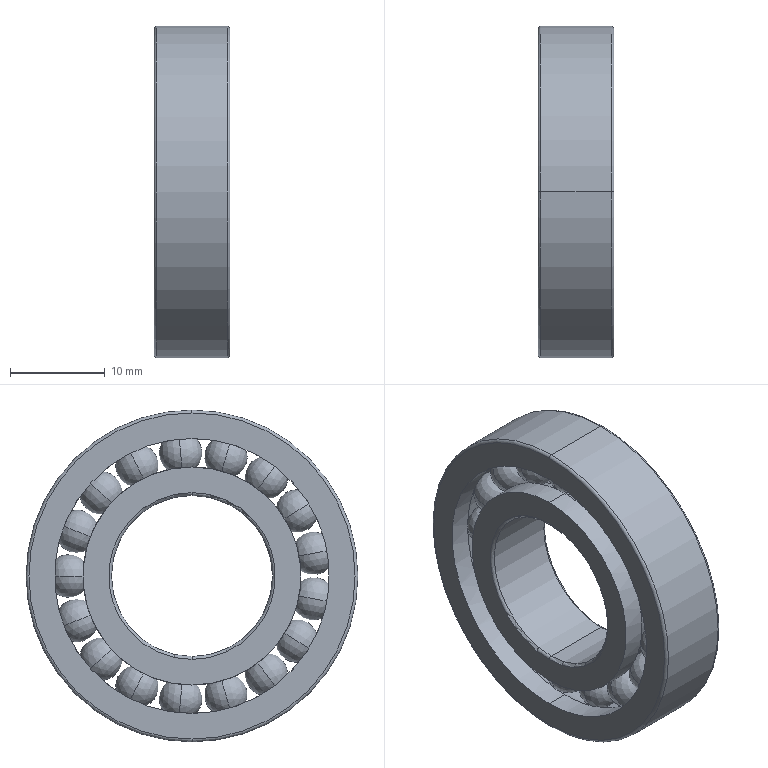Part | SolidWorks | features MoveCopyBody 1, Stock 1 | 1 solid | 112 faces | box 8 x 35 x 35 mm | volume 4447 mm3 | torus 62 | sphere 34 | cylinder 12 | plane 4 | commonest cylinder face diameters 23 x4 29 x4 17 x2 35 x2